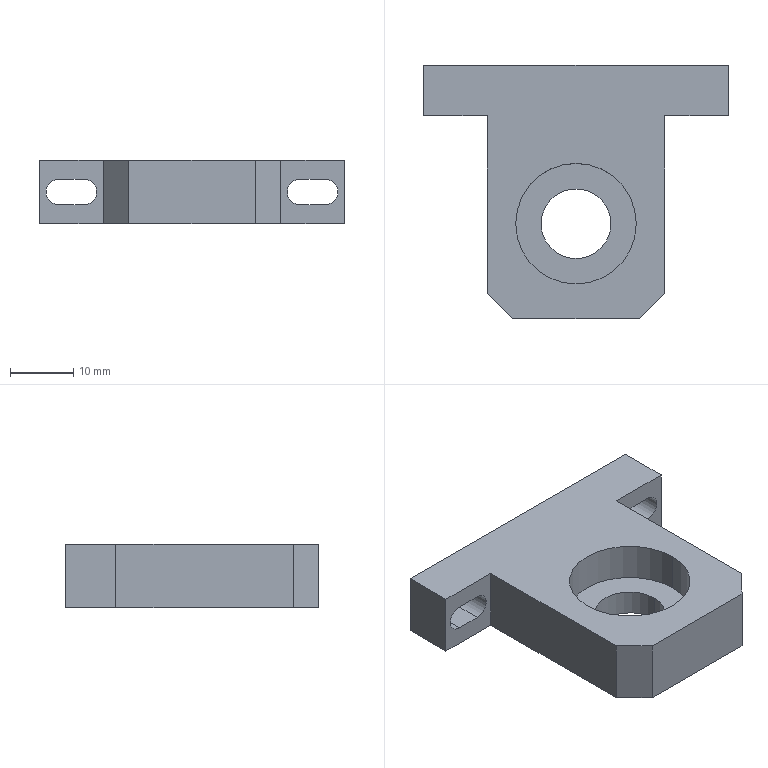Part | SolidWorks | features BaseBody 1 | 1 solid | 25 faces | box 48 x 40 x 10 mm | volume 10102 mm3 | plane 17 | cylinder 8 | commonest cylinder face diameters 4 x4 11 x2 19 x2
STEP:
#1=CARTESIAN_POINT('',(277.492,-152.944,0.));
#2=VERTEX_POINT('',#1);
#3=CARTESIAN_POINT('',(266.492,-152.944,0.));
#4=VERTEX_POINT('',#3);
#5=CARTESIAN_POINT('',(271.992,-152.944,0.));
#6=DIRECTION('',(0.,0.,-1.));
#7=DIRECTION('',(1.,0.,0.));
#8=AXIS2_PLACEMENT_3D('',#5,#6,#7);
#9=CIRCLE('',#8,5.5);
#10=EDGE_CURVE('',#2,#4,#9,.T.);
#11=ORIENTED_EDGE('',*,*,#10,.T.);
#12=CARTESIAN_POINT('',(266.492,-152.944,4.));
#13=VERTEX_POINT('',#12);
#14=CARTESIAN_POINT('',(266.492,-152.944,-47.446));
#15=DIRECTION('',(0.,0.,1.));
#16=VECTOR('',#15,1000.);
#17=LINE('',#14,#16);
#18=EDGE_CURVE('',#4,#13,#17,.T.);
#19=ORIENTED_EDGE('',*,*,#18,.T.);
#20=CARTESIAN_POINT('',(277.492,-152.944,4.));
#21=VERTEX_POINT('',#20);
#22=CARTESIAN_POINT('',(271.992,-152.944,4.));
#23=DIRECTION('',(0.,0.,-1.));
#24=DIRECTION('',(1.,0.,0.));
#25=AXIS2_PLACEMENT_3D('',#22,#23,#24);
#26=CIRCLE('',#25,5.5);
#27=EDGE_CURVE('',#21,#13,#26,.T.);
#28=ORIENTED_EDGE('',*,*,#27,.F.);
#29=CARTESIAN_POINT('',(277.492,-152.944,-47.446));
#30=DIRECTION('',(0.,0.,1.));
#31=VECTOR('',#30,1000.);
#32=LINE('',#29,#31);
#33=EDGE_CURVE('',#2,#21,#32,.T.);
#34=ORIENTED_EDGE('',*,*,#33,.F.);
#35=EDGE_LOOP('',(#11,#19,#28,#34));
#36=FACE_OUTER_BOUND('',#35,.T.);
#37=CARTESIAN_POINT('',(271.992,-152.944,-47.446));
#38=DIRECTION('',(0.,0.,1.));
#39=DIRECTION('',(1.,0.,0.));
#40=AXIS2_PLACEMENT_3D('',#37,#38,#39);
#41=CYLINDRICAL_SURFACE('',#40,5.5);
#42=ADVANCED_FACE('',(#36),#41,.F.);
#43=CARTESIAN_POINT('',(262.492,-152.944,4.));
#44=VERTEX_POINT('',#43);
#45=CARTESIAN_POINT('',(281.492,-152.944,4.));
#46=VERTEX_POINT('',#45);
#47=CARTESIAN_POINT('',(271.992,-152.944,4.));
#48=DIRECTION('',(0.,0.,1.));
#49=DIRECTION('',(1.,0.,0.));
#50=AXIS2_PLACEMENT_3D('',#47,#48,#49);
#51=CIRCLE('',#50,9.5);
#52=EDGE_CURVE('',#44,#46,#51,.T.);
#53=ORIENTED_EDGE('',*,*,#52,.F.);
#54=CARTESIAN_POINT('',(262.492,-152.944,10.));
#55=VERTEX_POINT('',#54);
#56=CARTESIAN_POINT('',(262.492,-152.944,7.));
#57=DIRECTION('',(0.,0.,1.));
#58=VECTOR('',#57,1000.);
#59=LINE('',#56,#58);
#60=EDGE_CURVE('',#44,#55,#59,.T.);
#61=ORIENTED_EDGE('',*,*,#60,.T.);
#62=CARTESIAN_POINT('',(281.492,-152.944,10.));
#63=VERTEX_POINT('',#62);
#64=CARTESIAN_POINT('',(271.992,-152.944,10.));
#65=DIRECTION('',(0.,0.,-1.));
#66=DIRECTION('',(1.,0.,0.));
#67=AXIS2_PLACEMENT_3D('',#64,#65,#66);
#68=CIRCLE('',#67,9.5);
#69=EDGE_CURVE('',#63,#55,#68,.T.);
#70=ORIENTED_EDGE('',*,*,#69,.F.);
#71=CARTESIAN_POINT('',(281.492,-152.944,7.));
#72=DIRECTION('',(0.,0.,1.));
#73=VECTOR('',#72,1000.);
#74=LINE('',#71,#73);
#75=EDGE_CURVE('',#46,#63,#74,.T.);
#76=ORIENTED_EDGE('',*,*,#75,.F.);
#77=EDGE_LOOP('',(#53,#61,#70,#76));
#78=FACE_OUTER_BOUND('',#77,.T.);
#79=CARTESIAN_POINT('',(271.992,-152.944,7.));
#80=DIRECTION('',(0.,0.,1.));
#81=DIRECTION('',(1.,0.,0.));
#82=AXIS2_PLACEMENT_3D('',#79,#80,#81);
#83=CYLINDRICAL_SURFACE('',#82,9.5);
#84=ADVANCED_FACE('',(#78),#83,.F.);
#85=ORIENTED_EDGE('',*,*,#10,.F.);
#86=CARTESIAN_POINT('',(271.992,-152.944,0.));
#87=DIRECTION('',(0.,0.,-1.));
#88=DIRECTION('',(1.,0.,0.));
#89=AXIS2_PLACEMENT_3D('',#86,#87,#88);
#90=CIRCLE('',#89,5.5);
#91=EDGE_CURVE('',#4,#2,#90,.T.);
#92=ORIENTED_EDGE('',*,*,#91,.F.);
#93=EDGE_LOOP('',(#85,#92));
#94=FACE_BOUND('',#93,.T.);
#95=CARTESIAN_POINT('',(261.992,-167.944,0.));
#96=VERTEX_POINT('',#95);
#97=CARTESIAN_POINT('',(281.992,-167.944,0.));
#98=VERTEX_POINT('',#97);
#99=CARTESIAN_POINT('',(271.992,-167.944,0.));
#100=DIRECTION('',(1.,0.,0.));
#101=VECTOR('',#100,1000.);
#102=LINE('',#99,#101);
#103=EDGE_CURVE('',#96,#98,#102,.T.);
#104=ORIENTED_EDGE('',*,*,#103,.F.);
#105=CARTESIAN_POINT('',(257.992,-163.944,0.));
#106=VERTEX_POINT('',#105);
#107=CARTESIAN_POINT('',(257.992,-163.944,0.));
#108=DIRECTION('',(0.7071,-0.7071,0.));
#109=VECTOR('',#108,1000.);
#110=LINE('',#107,#109);
#111=EDGE_CURVE('',#106,#96,#110,.T.);
#112=ORIENTED_EDGE('',*,*,#111,.F.);
#113=CARTESIAN_POINT('',(257.992,-135.944,0.));
#114=VERTEX_POINT('',#113);
#115=CARTESIAN_POINT('',(257.992,-147.944,0.));
#116=DIRECTION('',(0.,-1.,0.));
#117=VECTOR('',#116,1000.);
#118=LINE('',#115,#117);
#119=EDGE_CURVE('',#114,#106,#118,.T.);
#120=ORIENTED_EDGE('',*,*,#119,.F.);
#121=CARTESIAN_POINT('',(247.992,-135.944,0.));
#122=VERTEX_POINT('',#121);
#123=CARTESIAN_POINT('',(271.992,-135.944,0.));
#124=DIRECTION('',(1.,0.,0.));
#125=VECTOR('',#124,1000.);
#126=LINE('',#123,#125);
#127=EDGE_CURVE('',#122,#114,#126,.T.);
#128=ORIENTED_EDGE('',*,*,#127,.F.);
#129=CARTESIAN_POINT('',(247.992,-127.944,0.));
#130=VERTEX_POINT('',#129);
#131=CARTESIAN_POINT('',(247.992,-147.944,0.));
#132=DIRECTION('',(0.,-1.,0.));
#133=VECTOR('',#132,1000.);
#134=LINE('',#131,#133);
#135=EDGE_CURVE('',#130,#122,#134,.T.);
#136=ORIENTED_EDGE('',*,*,#135,.F.);
#137=CARTESIAN_POINT('',(295.992,-127.944,0.));
#138=VERTEX_POINT('',#137);
#139=CARTESIAN_POINT('',(271.992,-127.944,0.));
#140=DIRECTION('',(-1.,0.,0.));
#141=VECTOR('',#140,1000.);
#142=LINE('',#139,#141);
#143=EDGE_CURVE('',#138,#130,#142,.T.);
#144=ORIENTED_EDGE('',*,*,#143,.F.);
#145=CARTESIAN_POINT('',(295.992,-135.944,0.));
#146=VERTEX_POINT('',#145);
#147=CARTESIAN_POINT('',(295.992,-147.944,0.));
#148=DIRECTION('',(0.,1.,0.));
#149=VECTOR('',#148,1000.);
#150=LINE('',#147,#149);
#151=EDGE_CURVE('',#146,#138,#150,.T.);
#152=ORIENTED_EDGE('',*,*,#151,.F.);
#153=CARTESIAN_POINT('',(285.992,-135.944,0.));
#154=VERTEX_POINT('',#153);
#155=CARTESIAN_POINT('',(271.992,-135.944,0.));
#156=DIRECTION('',(1.,0.,0.));
#157=VECTOR('',#156,1000.);
#158=LINE('',#155,#157);
#159=EDGE_CURVE('',#154,#146,#158,.T.);
#160=ORIENTED_EDGE('',*,*,#159,.F.);
#161=CARTESIAN_POINT('',(285.992,-163.944,0.));
#162=VERTEX_POINT('',#161);
#163=CARTESIAN_POINT('',(285.992,-147.944,0.));
#164=DIRECTION('',(0.,1.,0.));
#165=VECTOR('',#164,1000.);
#166=LINE('',#163,#165);
#167=EDGE_CURVE('',#162,#154,#166,.T.);
#168=ORIENTED_EDGE('',*,*,#167,.F.);
#169=CARTESIAN_POINT('',(281.992,-167.944,0.));
#170=DIRECTION('',(0.7071,0.7071,0.));
#171=VECTOR('',#170,1000.);
#172=LINE('',#169,#171);
#173=EDGE_CURVE('',#98,#162,#172,.T.);
#174=ORIENTED_EDGE('',*,*,#173,.F.);
#175=EDGE_LOOP('',(#104,#112,#120,#128,#136,#144,#152,#160,#168,#174));
#176=FACE_OUTER_BOUND('',#175,.T.);
#177=CARTESIAN_POINT('',(271.992,-147.944,0.));
#178=DIRECTION('',(0.,0.,1.));
#179=DIRECTION('',(1.,0.,0.));
#180=AXIS2_PLACEMENT_3D('',#177,#178,#179);
#181=PLANE('',#180);
#182=ADVANCED_FACE('',(#94,#176),#181,.F.);
#183=ORIENTED_EDGE('',*,*,#18,.F.);
#184=ORIENTED_EDGE('',*,*,#91,.T.);
#185=ORIENTED_EDGE('',*,*,#33,.T.);
#186=CARTESIAN_POINT('',(271.992,-152.944,4.));
#187=DIRECTION('',(0.,0.,-1.));
#188=DIRECTION('',(1.,0.,0.));
#189=AXIS2_PLACEMENT_3D('',#186,#187,#188);
#190=CIRCLE('',#189,5.5);
#191=EDGE_CURVE('',#13,#21,#190,.T.);
#192=ORIENTED_EDGE('',*,*,#191,.F.);
#193=EDGE_LOOP('',(#183,#184,#185,#192));
#194=FACE_OUTER_BOUND('',#193,.T.);
#195=CARTESIAN_POINT('',(271.992,-152.944,-47.446));
#196=DIRECTION('',(0.,0.,1.));
#197=DIRECTION('',(1.,0.,0.));
#198=AXIS2_PLACEMENT_3D('',#195,#196,#197);
#199=CYLINDRICAL_SURFACE('',#198,5.5);
#200=ADVANCED_FACE('',(#194),#199,.F.);
#201=ORIENTED_EDGE('',*,*,#173,.T.);
#202=CARTESIAN_POINT('',(285.992,-163.944,10.));
#203=VERTEX_POINT('',#202);
#204=CARTESIAN_POINT('',(285.992,-163.944,5.));
#205=DIRECTION('',(0.,0.,1.));
#206=VECTOR('',#205,1000.);
#207=LINE('',#204,#206);
#208=EDGE_CURVE('',#162,#203,#207,.T.);
#209=ORIENTED_EDGE('',*,*,#208,.T.);
#210=CARTESIAN_POINT('',(281.992,-167.944,10.));
#211=VERTEX_POINT('',#210);
#212=CARTESIAN_POINT('',(283.992,-165.944,10.));
#213=DIRECTION('',(-0.7071,-0.7071,0.));
#214=VECTOR('',#213,1000.);
#215=LINE('',#212,#214);
#216=EDGE_CURVE('',#203,#211,#215,.T.);
#217=ORIENTED_EDGE('',*,*,#216,.T.);
#218=CARTESIAN_POINT('',(281.992,-167.944,5.));
#219=DIRECTION('',(0.,0.,-1.));
#220=VECTOR('',#219,1000.);
#221=LINE('',#218,#220);
#222=EDGE_CURVE('',#211,#98,#221,.T.);
#223=ORIENTED_EDGE('',*,*,#222,.T.);
#224=EDGE_LOOP('',(#201,#209,#217,#223));
#225=FACE_OUTER_BOUND('',#224,.T.);
#226=CARTESIAN_POINT('',(283.992,-165.944,5.));
#227=DIRECTION('',(0.7071,-0.7071,0.));
#228=DIRECTION('',(0.7071,0.7071,0.));
#229=AXIS2_PLACEMENT_3D('',#226,#227,#228);
#230=PLANE('',#229);
#231=ADVANCED_FACE('',(#225),#230,.T.);
#232=CARTESIAN_POINT('',(261.992,-167.944,10.));
#233=VERTEX_POINT('',#232);
#234=CARTESIAN_POINT('',(261.992,-167.944,0.));
#235=DIRECTION('',(0.,0.,-1.));
#236=VECTOR('',#235,1000.);
#237=LINE('',#234,#236);
#238=EDGE_CURVE('',#233,#96,#237,.T.);
#239=ORIENTED_EDGE('',*,*,#238,.T.);
#240=ORIENTED_EDGE('',*,*,#103,.T.);
#241=ORIENTED_EDGE('',*,*,#222,.F.);
#242=CARTESIAN_POINT('',(291.992,-167.944,10.));
#243=DIRECTION('',(-1.,0.,0.));
#244=VECTOR('',#243,1000.);
#245=LINE('',#242,#244);
#246=EDGE_CURVE('',#211,#233,#245,.T.);
#247=ORIENTED_EDGE('',*,*,#246,.T.);
#248=EDGE_LOOP('',(#239,#240,#241,#247));
#249=FACE_OUTER_BOUND('',#248,.T.);
#250=CARTESIAN_POINT('',(291.992,-167.944,0.));
#251=DIRECTION('',(0.,-1.,0.));
#252=DIRECTION('',(0.,0.,-1.));
#253=AXIS2_PLACEMENT_3D('',#250,#251,#252);
#254=PLANE('',#253);
#255=ADVANCED_FACE('',(#249),#254,.T.);
#256=CARTESIAN_POINT('',(257.992,-163.944,10.));
#257=VERTEX_POINT('',#256);
#258=CARTESIAN_POINT('',(259.992,-165.944,10.));
#259=DIRECTION('',(-0.7071,0.7071,0.));
#260=VECTOR('',#259,1000.);
#261=LINE('',#258,#260);
#262=EDGE_CURVE('',#233,#257,#261,.T.);
#263=ORIENTED_EDGE('',*,*,#262,.T.);
#264=CARTESIAN_POINT('',(257.992,-163.944,5.));
#265=DIRECTION('',(0.,0.,-1.));
#266=VECTOR('',#265,1000.);
#267=LINE('',#264,#266);
#268=EDGE_CURVE('',#257,#106,#267,.T.);
#269=ORIENTED_EDGE('',*,*,#268,.T.);
#270=ORIENTED_EDGE('',*,*,#111,.T.);
#271=ORIENTED_EDGE('',*,*,#238,.F.);
#272=EDGE_LOOP('',(#263,#269,#270,#271));
#273=FACE_OUTER_BOUND('',#272,.T.);
#274=CARTESIAN_POINT('',(259.992,-165.944,5.));
#275=DIRECTION('',(-0.7071,-0.7071,0.));
#276=DIRECTION('',(0.7071,-0.7071,0.));
#277=AXIS2_PLACEMENT_3D('',#274,#275,#276);
#278=PLANE('',#277);
#279=ADVANCED_FACE('',(#273),#278,.T.);
#280=CARTESIAN_POINT('',(257.992,-135.944,10.));
#281=VERTEX_POINT('',#280);
#282=CARTESIAN_POINT('',(257.992,-167.944,10.));
#283=DIRECTION('',(0.,-1.,0.));
#284=VECTOR('',#283,1000.);
#285=LINE('',#282,#284);
#286=EDGE_CURVE('',#281,#257,#285,.T.);
#287=ORIENTED_EDGE('',*,*,#286,.F.);
#288=CARTESIAN_POINT('',(257.992,-135.944,10.));
#289=DIRECTION('',(0.,0.,1.));
#290=VECTOR('',#289,1000.);
#291=LINE('',#288,#290);
#292=EDGE_CURVE('',#114,#281,#291,.T.);
#293=ORIENTED_EDGE('',*,*,#292,.F.);
#294=ORIENTED_EDGE('',*,*,#119,.T.);
#295=ORIENTED_EDGE('',*,*,#268,.F.);
#296=EDGE_LOOP('',(#287,#293,#294,#295));
#297=FACE_OUTER_BOUND('',#296,.T.);
#298=CARTESIAN_POINT('',(257.992,-167.944,10.));
#299=DIRECTION('',(1.,0.,0.));
#300=DIRECTION('',(0.,0.,-1.));
#301=AXIS2_PLACEMENT_3D('',#298,#299,#300);
#302=PLANE('',#301);
#303=ADVANCED_FACE('',(#297),#302,.F.);
#304=CARTESIAN_POINT('',(250.992,-135.944,3.));
#305=VERTEX_POINT('',#304);
#306=CARTESIAN_POINT('',(254.992,-135.944,3.));
#307=VERTEX_POINT('',#306);
#308=CARTESIAN_POINT('',(257.992,-135.944,3.));
#309=DIRECTION('',(1.,0.,0.));
#310=VECTOR('',#309,1000.);
#311=LINE('',#308,#310);
#312=EDGE_CURVE('',#305,#307,#311,.T.);
#313=ORIENTED_EDGE('',*,*,#312,.F.);
#314=CARTESIAN_POINT('',(250.992,-135.944,7.));
#315=VERTEX_POINT('',#314);
#316=CARTESIAN_POINT('',(250.992,-135.944,5.));
#317=DIRECTION('',(0.,-1.,0.));
#318=DIRECTION('',(0.,0.,1.));
#319=AXIS2_PLACEMENT_3D('',#316,#317,#318);
#320=CIRCLE('',#319,2.);
#321=EDGE_CURVE('',#315,#305,#320,.T.);
#322=ORIENTED_EDGE('',*,*,#321,.F.);
#323=CARTESIAN_POINT('',(254.992,-135.944,7.));
#324=VERTEX_POINT('',#323);
#325=CARTESIAN_POINT('',(257.992,-135.944,7.));
#326=DIRECTION('',(-1.,0.,0.));
#327=VECTOR('',#326,1000.);
#328=LINE('',#325,#327);
#329=EDGE_CURVE('',#324,#315,#328,.T.);
#330=ORIENTED_EDGE('',*,*,#329,.F.);
#331=CARTESIAN_POINT('',(254.992,-135.944,5.));
#332=DIRECTION('',(0.,-1.,0.));
#333=DIRECTION('',(0.,0.,1.));
#334=AXIS2_PLACEMENT_3D('',#331,#332,#333);
#335=CIRCLE('',#334,2.);
#336=EDGE_CURVE('',#307,#324,#335,.T.);
#337=ORIENTED_EDGE('',*,*,#336,.F.);
#338=EDGE_LOOP('',(#313,#322,#330,#337));
#339=FACE_BOUND('',#338,.T.);
#340=ORIENTED_EDGE('',*,*,#292,.T.);
#341=CARTESIAN_POINT('',(247.992,-135.944,10.));
#342=VERTEX_POINT('',#341);
#343=CARTESIAN_POINT('',(257.992,-135.944,10.));
#344=DIRECTION('',(1.,0.,0.));
#345=VECTOR('',#344,1000.);
#346=LINE('',#343,#345);
#347=EDGE_CURVE('',#342,#281,#346,.T.);
#348=ORIENTED_EDGE('',*,*,#347,.F.);
#349=CARTESIAN_POINT('',(247.992,-135.944,10.));
#350=DIRECTION('',(0.,0.,1.));
#351=VECTOR('',#350,1000.);
#352=LINE('',#349,#351);
#353=EDGE_CURVE('',#122,#342,#352,.T.);
#354=ORIENTED_EDGE('',*,*,#353,.F.);
#355=ORIENTED_EDGE('',*,*,#127,.T.);
#356=EDGE_LOOP('',(#340,#348,#354,#355));
#357=FACE_OUTER_BOUND('',#356,.T.);
#358=CARTESIAN_POINT('',(257.992,-135.944,10.));
#359=DIRECTION('',(0.,1.,0.));
#360=DIRECTION('',(0.,0.,1.));
#361=AXIS2_PLACEMENT_3D('',#358,#359,#360);
#362=PLANE('',#361);
#363=ADVANCED_FACE('',(#339,#357),#362,.F.);
#364=ORIENTED_EDGE('',*,*,#353,.T.);
#365=CARTESIAN_POINT('',(247.992,-127.944,10.));
#366=VERTEX_POINT('',#365);
#367=CARTESIAN_POINT('',(247.992,-131.944,10.));
#368=DIRECTION('',(0.,-1.,0.));
#369=VECTOR('',#368,1000.);
#370=LINE('',#367,#369);
#371=EDGE_CURVE('',#366,#342,#370,.T.);
#372=ORIENTED_EDGE('',*,*,#371,.F.);
#373=CARTESIAN_POINT('',(247.992,-127.944,5.));
#374=DIRECTION('',(0.,0.,1.));
#375=VECTOR('',#374,1000.);
#376=LINE('',#373,#375);
#377=EDGE_CURVE('',#130,#366,#376,.T.);
#378=ORIENTED_EDGE('',*,*,#377,.F.);
#379=ORIENTED_EDGE('',*,*,#135,.T.);
#380=EDGE_LOOP('',(#364,#372,#378,#379));
#381=FACE_OUTER_BOUND('',#380,.T.);
#382=CARTESIAN_POINT('',(247.992,-131.944,5.));
#383=DIRECTION('',(1.,0.,0.));
#384=DIRECTION('',(0.,0.,-1.));
#385=AXIS2_PLACEMENT_3D('',#382,#383,#384);
#386=PLANE('',#385);
#387=ADVANCED_FACE('',(#381),#386,.F.);
#388=CARTESIAN_POINT('',(250.992,-127.944,7.));
#389=VERTEX_POINT('',#388);
#390=CARTESIAN_POINT('',(250.992,-127.944,3.));
#391=VERTEX_POINT('',#390);
#392=CARTESIAN_POINT('',(250.992,-127.944,5.));
#393=DIRECTION('',(0.,-1.,0.));
#394=DIRECTION('',(0.,0.,1.));
#395=AXIS2_PLACEMENT_3D('',#392,#393,#394);
#396=CIRCLE('',#395,2.);
#397=EDGE_CURVE('',#389,#391,#396,.T.);
#398=ORIENTED_EDGE('',*,*,#397,.T.);
#399=CARTESIAN_POINT('',(254.992,-127.944,3.));
#400=VERTEX_POINT('',#399);
#401=CARTESIAN_POINT('',(251.992,-127.944,3.));
#402=DIRECTION('',(1.,0.,0.));
#403=VECTOR('',#402,1000.);
#404=LINE('',#401,#403);
#405=EDGE_CURVE('',#391,#400,#404,.T.);
#406=ORIENTED_EDGE('',*,*,#405,.T.);
#407=CARTESIAN_POINT('',(254.992,-127.944,7.));
#408=VERTEX_POINT('',#407);
#409=CARTESIAN_POINT('',(254.992,-127.944,5.));
#410=DIRECTION('',(0.,-1.,0.));
#411=DIRECTION('',(0.,0.,1.));
#412=AXIS2_PLACEMENT_3D('',#409,#410,#411);
#413=CIRCLE('',#412,2.);
#414=EDGE_CURVE('',#400,#408,#413,.T.);
#415=ORIENTED_EDGE('',*,*,#414,.T.);
#416=CARTESIAN_POINT('',(251.992,-127.944,7.));
#417=DIRECTION('',(-1.,0.,0.));
#418=VECTOR('',#417,1000.);
#419=LINE('',#416,#418);
#420=EDGE_CURVE('',#408,#389,#419,.T.);
#421=ORIENTED_EDGE('',*,*,#420,.T.);
#422=EDGE_LOOP('',(#398,#406,#415,#421));
#423=FACE_BOUND('',#422,.T.);
#424=CARTESIAN_POINT('',(288.992,-127.944,7.));
#425=VERTEX_POINT('',#424);
#426=CARTESIAN_POINT('',(288.992,-127.944,3.));
#427=VERTEX_POINT('',#426);
#428=CARTESIAN_POINT('',(288.992,-127.944,5.));
#429=DIRECTION('',(0.,-1.,0.));
#430=DIRECTION('',(0.,0.,1.));
#431=AXIS2_PLACEMENT_3D('',#428,#429,#430);
#432=CIRCLE('',#431,2.);
#433=EDGE_CURVE('',#425,#427,#432,.T.);
#434=ORIENTED_EDGE('',*,*,#433,.T.);
#435=CARTESIAN_POINT('',(292.992,-127.944,3.));
#436=VERTEX_POINT('',#435);
#437=CARTESIAN_POINT('',(251.992,-127.944,3.));
#438=DIRECTION('',(1.,0.,0.));
#439=VECTOR('',#438,1000.);
#440=LINE('',#437,#439);
#441=EDGE_CURVE('',#427,#436,#440,.T.);
#442=ORIENTED_EDGE('',*,*,#441,.T.);
#443=CARTESIAN_POINT('',(292.992,-127.944,7.));
#444=VERTEX_POINT('',#443);
#445=CARTESIAN_POINT('',(292.992,-127.944,5.));
#446=DIRECTION('',(0.,-1.,0.));
#447=DIRECTION('',(0.,0.,1.));
#448=AXIS2_PLACEMENT_3D('',#445,#446,#447);
#449=CIRCLE('',#448,2.);
#450=EDGE_CURVE('',#436,#444,#449,.T.);
#451=ORIENTED_EDGE('',*,*,#450,.T.);
#452=CARTESIAN_POINT('',(251.992,-127.944,7.));
#453=DIRECTION('',(-1.,0.,0.));
#454=VECTOR('',#453,1000.);
#455=LINE('',#452,#454);
#456=EDGE_CURVE('',#444,#425,#455,.T.);
#457=ORIENTED_EDGE('',*,*,#456,.T.);
#458=EDGE_LOOP('',(#434,#442,#451,#457));
#459=FACE_BOUND('',#458,.T.);
#460=ORIENTED_EDGE('',*,*,#143,.T.);
#461=ORIENTED_EDGE('',*,*,#377,.T.);
#462=CARTESIAN_POINT('',(295.992,-127.944,10.));
#463=VERTEX_POINT('',#462);
#464=CARTESIAN_POINT('',(251.992,-127.944,10.));
#465=DIRECTION('',(1.,0.,0.));
#466=VECTOR('',#465,1000.);
#467=LINE('',#464,#466);
#468=EDGE_CURVE('',#366,#463,#467,.T.);
#469=ORIENTED_EDGE('',*,*,#468,.T.);
#470=CARTESIAN_POINT('',(295.992,-127.944,0.));
#471=DIRECTION('',(0.,0.,-1.));
#472=VECTOR('',#471,1000.);
#473=LINE('',#470,#472);
#474=EDGE_CURVE('',#463,#138,#473,.T.);
#475=ORIENTED_EDGE('',*,*,#474,.T.);
#476=EDGE_LOOP('',(#460,#461,#469,#475));
#477=FACE_OUTER_BOUND('',#476,.T.);
#478=CARTESIAN_POINT('',(251.992,-127.944,0.));
#479=DIRECTION('',(0.,1.,0.));
#480=DIRECTION('',(0.,0.,1.));
#481=AXIS2_PLACEMENT_3D('',#478,#479,#480);
#482=PLANE('',#481);
#483=ADVANCED_FACE('',(#423,#459,#477),#482,.T.);
#484=ORIENTED_EDGE('',*,*,#151,.T.);
#485=ORIENTED_EDGE('',*,*,#474,.F.);
#486=CARTESIAN_POINT('',(295.992,-135.944,10.));
#487=VERTEX_POINT('',#486);
#488=CARTESIAN_POINT('',(295.992,-131.944,10.));
#489=DIRECTION('',(0.,-1.,0.));
#490=VECTOR('',#489,1000.);
#491=LINE('',#488,#490);
#492=EDGE_CURVE('',#463,#487,#491,.T.);
#493=ORIENTED_EDGE('',*,*,#492,.T.);
#494=CARTESIAN_POINT('',(295.992,-135.944,5.));
#495=DIRECTION('',(0.,0.,-1.));
#496=VECTOR('',#495,1000.);
#497=LINE('',#494,#496);
#498=EDGE_CURVE('',#487,#146,#497,.T.);
#499=ORIENTED_EDGE('',*,*,#498,.T.);
#500=EDGE_LOOP('',(#484,#485,#493,#499));
#501=FACE_OUTER_BOUND('',#500,.T.);
#502=CARTESIAN_POINT('',(295.992,-131.944,5.));
#503=DIRECTION('',(1.,0.,0.));
#504=DIRECTION('',(0.,0.,-1.));
#505=AXIS2_PLACEMENT_3D('',#502,#503,#504);
#506=PLANE('',#505);
#507=ADVANCED_FACE('',(#501),#506,.T.);
#508=CARTESIAN_POINT('',(288.992,-135.944,3.));
#509=VERTEX_POINT('',#508);
#510=CARTESIAN_POINT('',(292.992,-135.944,3.));
#511=VERTEX_POINT('',#510);
#512=CARTESIAN_POINT('',(291.992,-135.944,3.));
#513=DIRECTION('',(1.,0.,0.));
#514=VECTOR('',#513,1000.);
#515=LINE('',#512,#514);
#516=EDGE_CURVE('',#509,#511,#515,.T.);
#517=ORIENTED_EDGE('',*,*,#516,.F.);
#518=CARTESIAN_POINT('',(288.992,-135.944,7.));
#519=VERTEX_POINT('',#518);
#520=CARTESIAN_POINT('',(288.992,-135.944,5.));
#521=DIRECTION('',(0.,-1.,0.));
#522=DIRECTION('',(0.,0.,1.));
#523=AXIS2_PLACEMENT_3D('',#520,#521,#522);
#524=CIRCLE('',#523,2.);
#525=EDGE_CURVE('',#519,#509,#524,.T.);
#526=ORIENTED_EDGE('',*,*,#525,.F.);
#527=CARTESIAN_POINT('',(292.992,-135.944,7.));
#528=VERTEX_POINT('',#527);
#529=CARTESIAN_POINT('',(291.992,-135.944,7.));
#530=DIRECTION('',(-1.,0.,0.));
#531=VECTOR('',#530,1000.);
#532=LINE('',#529,#531);
#533=EDGE_CURVE('',#528,#519,#532,.T.);
#534=ORIENTED_EDGE('',*,*,#533,.F.);
#535=CARTESIAN_POINT('',(292.992,-135.944,5.));
#536=DIRECTION('',(0.,-1.,0.));
#537=DIRECTION('',(0.,0.,1.));
#538=AXIS2_PLACEMENT_3D('',#535,#536,#537);
#539=CIRCLE('',#538,2.);
#540=EDGE_CURVE('',#511,#528,#539,.T.);
#541=ORIENTED_EDGE('',*,*,#540,.F.);
#542=EDGE_LOOP('',(#517,#526,#534,#541));
#543=FACE_BOUND('',#542,.T.);
#544=ORIENTED_EDGE('',*,*,#498,.F.);
#545=CARTESIAN_POINT('',(285.992,-135.944,10.));
#546=VERTEX_POINT('',#545);
#547=CARTESIAN_POINT('',(291.992,-135.944,10.));
#548=DIRECTION('',(1.,0.,0.));
#549=VECTOR('',#548,1000.);
#550=LINE('',#547,#549);
#551=EDGE_CURVE('',#546,#487,#550,.T.);
#552=ORIENTED_EDGE('',*,*,#551,.F.);
#553=CARTESIAN_POINT('',(285.992,-135.944,10.));
#554=DIRECTION('',(0.,0.,1.));
#555=VECTOR('',#554,1000.);
#556=LINE('',#553,#555);
#557=EDGE_CURVE('',#154,#546,#556,.T.);
#558=ORIENTED_EDGE('',*,*,#557,.F.);
#559=ORIENTED_EDGE('',*,*,#159,.T.);
#560=EDGE_LOOP('',(#544,#552,#558,#559));
#561=FACE_OUTER_BOUND('',#560,.T.);
#562=CARTESIAN_POINT('',(291.992,-135.944,10.));
#563=DIRECTION('',(0.,1.,0.));
#564=DIRECTION('',(0.,0.,1.));
#565=AXIS2_PLACEMENT_3D('',#562,#563,#564);
#566=PLANE('',#565);
#567=ADVANCED_FACE('',(#543,#561),#566,.F.);
#568=ORIENTED_EDGE('',*,*,#167,.T.);
#569=ORIENTED_EDGE('',*,*,#557,.T.);
#570=CARTESIAN_POINT('',(285.992,-135.944,10.));
#571=DIRECTION('',(0.,1.,0.));
#572=VECTOR('',#571,1000.);
#573=LINE('',#570,#572);
#574=EDGE_CURVE('',#203,#546,#573,.T.);
#575=ORIENTED_EDGE('',*,*,#574,.F.);
#576=ORIENTED_EDGE('',*,*,#208,.F.);
#577=EDGE_LOOP('',(#568,#569,#575,#576));
#578=FACE_OUTER_BOUND('',#577,.T.);
#579=CARTESIAN_POINT('',(285.992,-135.944,10.));
#580=DIRECTION('',(-1.,0.,0.));
#581=DIRECTION('',(0.,0.,1.));
#582=AXIS2_PLACEMENT_3D('',#579,#580,#581);
#583=PLANE('',#582);
#584=ADVANCED_FACE('',(#578),#583,.F.);
#585=ORIENTED_EDGE('',*,*,#27,.T.);
#586=ORIENTED_EDGE('',*,*,#191,.T.);
#587=EDGE_LOOP('',(#585,#586));
#588=FACE_BOUND('',#587,.T.);
#589=CARTESIAN_POINT('',(271.992,-152.944,4.));
#590=DIRECTION('',(0.,0.,1.));
#591=DIRECTION('',(1.,0.,0.));
#592=AXIS2_PLACEMENT_3D('',#589,#590,#591);
#593=CIRCLE('',#592,9.5);
#594=EDGE_CURVE('',#46,#44,#593,.T.);
#595=ORIENTED_EDGE('',*,*,#594,.T.);
#596=ORIENTED_EDGE('',*,*,#52,.T.);
#597=EDGE_LOOP('',(#595,#596));
#598=FACE_OUTER_BOUND('',#597,.T.);
#599=CARTESIAN_POINT('',(271.992,-152.944,4.));
#600=DIRECTION('',(0.,0.,1.));
#601=DIRECTION('',(1.,0.,0.));
#602=AXIS2_PLACEMENT_3D('',#599,#600,#601);
#603=PLANE('',#602);
#604=ADVANCED_FACE('',(#588,#598),#603,.T.);
#605=ORIENTED_EDGE('',*,*,#69,.T.);
#606=CARTESIAN_POINT('',(271.992,-152.944,10.));
#607=DIRECTION('',(0.,0.,-1.));
#608=DIRECTION('',(1.,0.,0.));
#609=AXIS2_PLACEMENT_3D('',#606,#607,#608);
#610=CIRCLE('',#609,9.5);
#611=EDGE_CURVE('',#55,#63,#610,.T.);
#612=ORIENTED_EDGE('',*,*,#611,.T.);
#613=EDGE_LOOP('',(#605,#612));
#614=FACE_BOUND('',#613,.T.);
#615=ORIENTED_EDGE('',*,*,#262,.F.);
#616=ORIENTED_EDGE('',*,*,#246,.F.);
#617=ORIENTED_EDGE('',*,*,#216,.F.);
#618=ORIENTED_EDGE('',*,*,#574,.T.);
#619=ORIENTED_EDGE('',*,*,#551,.T.);
#620=ORIENTED_EDGE('',*,*,#492,.F.);
#621=ORIENTED_EDGE('',*,*,#468,.F.);
#622=ORIENTED_EDGE('',*,*,#371,.T.);
#623=ORIENTED_EDGE('',*,*,#347,.T.);
#624=ORIENTED_EDGE('',*,*,#286,.T.);
#625=EDGE_LOOP('',(#615,#616,#617,#618,#619,#620,#621,#622,#623,#624));
#626=FACE_OUTER_BOUND('',#625,.T.);
#627=CARTESIAN_POINT('',(271.992,-147.944,10.));
#628=DIRECTION('',(0.,0.,1.));
#629=DIRECTION('',(1.,0.,0.));
#630=AXIS2_PLACEMENT_3D('',#627,#628,#629);
#631=PLANE('',#630);
#632=ADVANCED_FACE('',(#614,#626),#631,.T.);
#633=CARTESIAN_POINT('',(254.992,-135.944,3.));
#634=DIRECTION('',(0.,1.,0.));
#635=VECTOR('',#634,1000.);
#636=LINE('',#633,#635);
#637=EDGE_CURVE('',#307,#400,#636,.T.);
#638=ORIENTED_EDGE('',*,*,#637,.F.);
#639=ORIENTED_EDGE('',*,*,#336,.T.);
#640=CARTESIAN_POINT('',(254.992,-135.944,7.));
#641=DIRECTION('',(0.,-1.,0.));
#642=VECTOR('',#641,1000.);
#643=LINE('',#640,#642);
#644=EDGE_CURVE('',#408,#324,#643,.T.);
#645=ORIENTED_EDGE('',*,*,#644,.F.);
#646=ORIENTED_EDGE('',*,*,#414,.F.);
#647=EDGE_LOOP('',(#638,#639,#645,#646));
#648=FACE_OUTER_BOUND('',#647,.T.);
#649=CARTESIAN_POINT('',(254.992,-135.944,5.));
#650=DIRECTION('',(0.,1.,0.));
#651=DIRECTION('',(0.,0.,1.));
#652=AXIS2_PLACEMENT_3D('',#649,#650,#651);
#653=CYLINDRICAL_SURFACE('',#652,2.);
#654=ADVANCED_FACE('',(#648),#653,.F.);
#655=CARTESIAN_POINT('',(250.992,-135.944,3.));
#656=DIRECTION('',(0.,1.,0.));
#657=VECTOR('',#656,1000.);
#658=LINE('',#655,#657);
#659=EDGE_CURVE('',#305,#391,#658,.T.);
#660=ORIENTED_EDGE('',*,*,#659,.F.);
#661=ORIENTED_EDGE('',*,*,#312,.T.);
#662=ORIENTED_EDGE('',*,*,#637,.T.);
#663=ORIENTED_EDGE('',*,*,#405,.F.);
#664=EDGE_LOOP('',(#660,#661,#662,#663));
#665=FACE_OUTER_BOUND('',#664,.T.);
#666=CARTESIAN_POINT('',(250.992,-135.944,3.));
#667=DIRECTION('',(0.,0.,-1.));
#668=DIRECTION('',(-1.,0.,0.));
#669=AXIS2_PLACEMENT_3D('',#666,#667,#668);
#670=PLANE('',#669);
#671=ADVANCED_FACE('',(#665),#670,.F.);
#672=CARTESIAN_POINT('',(250.992,-135.944,7.));
#673=DIRECTION('',(0.,1.,0.));
#674=VECTOR('',#673,1000.);
#675=LINE('',#672,#674);
#676=EDGE_CURVE('',#315,#389,#675,.T.);
#677=ORIENTED_EDGE('',*,*,#676,.F.);
#678=ORIENTED_EDGE('',*,*,#321,.T.);
#679=ORIENTED_EDGE('',*,*,#659,.T.);
#680=ORIENTED_EDGE('',*,*,#397,.F.);
#681=EDGE_LOOP('',(#677,#678,#679,#680));
#682=FACE_OUTER_BOUND('',#681,.T.);
#683=CARTESIAN_POINT('',(250.992,-135.944,5.));
#684=DIRECTION('',(0.,1.,0.));
#685=DIRECTION('',(0.,0.,1.));
#686=AXIS2_PLACEMENT_3D('',#683,#684,#685);
#687=CYLINDRICAL_SURFACE('',#686,2.);
#688=ADVANCED_FACE('',(#682),#687,.F.);
#689=ORIENTED_EDGE('',*,*,#644,.T.);
#690=ORIENTED_EDGE('',*,*,#329,.T.);
#691=ORIENTED_EDGE('',*,*,#676,.T.);
#692=ORIENTED_EDGE('',*,*,#420,.F.);
#693=EDGE_LOOP('',(#689,#690,#691,#692));
#694=FACE_OUTER_BOUND('',#693,.T.);
#695=CARTESIAN_POINT('',(254.992,-135.944,7.));
#696=DIRECTION('',(0.,0.,1.));
#697=DIRECTION('',(1.,0.,0.));
#698=AXIS2_PLACEMENT_3D('',#695,#696,#697);
#699=PLANE('',#698);
#700=ADVANCED_FACE('',(#694),#699,.F.);
#701=CARTESIAN_POINT('',(288.992,-135.944,3.));
#702=DIRECTION('',(0.,1.,0.));
#703=VECTOR('',#702,1000.);
#704=LINE('',#701,#703);
#705=EDGE_CURVE('',#509,#427,#704,.T.);
#706=ORIENTED_EDGE('',*,*,#705,.F.);
#707=ORIENTED_EDGE('',*,*,#516,.T.);
#708=CARTESIAN_POINT('',(292.992,-135.944,3.));
#709=DIRECTION('',(0.,-1.,0.));
#710=VECTOR('',#709,1000.);
#711=LINE('',#708,#710);
#712=EDGE_CURVE('',#436,#511,#711,.T.);
#713=ORIENTED_EDGE('',*,*,#712,.F.);
#714=ORIENTED_EDGE('',*,*,#441,.F.);
#715=EDGE_LOOP('',(#706,#707,#713,#714));
#716=FACE_OUTER_BOUND('',#715,.T.);
#717=CARTESIAN_POINT('',(288.992,-135.944,3.));
#718=DIRECTION('',(0.,0.,-1.));
#719=DIRECTION('',(-1.,0.,0.));
#720=AXIS2_PLACEMENT_3D('',#717,#718,#719);
#721=PLANE('',#720);
#722=ADVANCED_FACE('',(#716),#721,.F.);
#723=CARTESIAN_POINT('',(288.992,-135.944,7.));
#724=DIRECTION('',(0.,1.,0.));
#725=VECTOR('',#724,1000.);
#726=LINE('',#723,#725);
#727=EDGE_CURVE('',#519,#425,#726,.T.);
#728=ORIENTED_EDGE('',*,*,#727,.F.);
#729=ORIENTED_EDGE('',*,*,#525,.T.);
#730=ORIENTED_EDGE('',*,*,#705,.T.);
#731=ORIENTED_EDGE('',*,*,#433,.F.);
#732=EDGE_LOOP('',(#728,#729,#730,#731));
#733=FACE_OUTER_BOUND('',#732,.T.);
#734=CARTESIAN_POINT('',(288.992,-135.944,5.));
#735=DIRECTION('',(0.,1.,0.));
#736=DIRECTION('',(0.,0.,1.));
#737=AXIS2_PLACEMENT_3D('',#734,#735,#736);
#738=CYLINDRICAL_SURFACE('',#737,2.);
#739=ADVANCED_FACE('',(#733),#738,.F.);
#740=CARTESIAN_POINT('',(292.992,-135.944,7.));
#741=DIRECTION('',(0.,1.,0.));
#742=VECTOR('',#741,1000.);
#743=LINE('',#740,#742);
#744=EDGE_CURVE('',#528,#444,#743,.T.);
#745=ORIENTED_EDGE('',*,*,#744,.F.);
#746=ORIENTED_EDGE('',*,*,#533,.T.);
#747=ORIENTED_EDGE('',*,*,#727,.T.);
#748=ORIENTED_EDGE('',*,*,#456,.F.);
#749=EDGE_LOOP('',(#745,#746,#747,#748));
#750=FACE_OUTER_BOUND('',#749,.T.);
#751=CARTESIAN_POINT('',(292.992,-135.944,7.));
#752=DIRECTION('',(0.,0.,1.));
#753=DIRECTION('',(1.,0.,0.));
#754=AXIS2_PLACEMENT_3D('',#751,#752,#753);
#755=PLANE('',#754);
#756=ADVANCED_FACE('',(#750),#755,.F.);
#757=ORIENTED_EDGE('',*,*,#712,.T.);
#758=ORIENTED_EDGE('',*,*,#540,.T.);
#759=ORIENTED_EDGE('',*,*,#744,.T.);
#760=ORIENTED_EDGE('',*,*,#450,.F.);
#761=EDGE_LOOP('',(#757,#758,#759,#760));
#762=FACE_OUTER_BOUND('',#761,.T.);
#763=CARTESIAN_POINT('',(292.992,-135.944,5.));
#764=DIRECTION('',(0.,1.,0.));
#765=DIRECTION('',(0.,0.,1.));
#766=AXIS2_PLACEMENT_3D('',#763,#764,#765);
#767=CYLINDRICAL_SURFACE('',#766,2.);
#768=ADVANCED_FACE('',(#762),#767,.F.);
#769=ORIENTED_EDGE('',*,*,#60,.F.);
#770=ORIENTED_EDGE('',*,*,#594,.F.);
#771=ORIENTED_EDGE('',*,*,#75,.T.);
#772=ORIENTED_EDGE('',*,*,#611,.F.);
#773=EDGE_LOOP('',(#769,#770,#771,#772));
#774=FACE_OUTER_BOUND('',#773,.T.);
#775=CARTESIAN_POINT('',(271.992,-152.944,7.));
#776=DIRECTION('',(0.,0.,1.));
#777=DIRECTION('',(1.,0.,0.));
#778=AXIS2_PLACEMENT_3D('',#775,#776,#777);
#779=CYLINDRICAL_SURFACE('',#778,9.5);
#780=ADVANCED_FACE('',(#774),#779,.F.);
#781=CLOSED_SHELL('',(#42,#84,#182,#200,#231,#255,#279,#303,#363,#387,#483,#507,#567,#584,#604,#632,#654,#671,#688,#700,#722,#739,#756,#768,#780));
#782=MANIFOLD_SOLID_BREP('',#781);
#783=CARTESIAN_POINT('',(0.,0.,0.));
#784=DIRECTION('',(0.,0.,1.));
#785=DIRECTION('',(1.,0.,0.));
#786=AXIS2_PLACEMENT_3D('',#783,#784,#785);
#787=(LENGTH_UNIT()NAMED_UNIT(*)SI_UNIT(.MILLI.,.METRE.));
#788=UNCERTAINTY_MEASURE_WITH_UNIT(LENGTH_MEASURE(0.00001),#787,'','');
#789=(NAMED_UNIT(*)PLANE_ANGLE_UNIT()SI_UNIT($,.RADIAN.));
#790=(NAMED_UNIT(*)SI_UNIT($,.STERADIAN.)SOLID_ANGLE_UNIT());
#791=(GEOMETRIC_REPRESENTATION_CONTEXT(3)GLOBAL_UNCERTAINTY_ASSIGNED_CONTEXT((#788))GLOBAL_UNIT_ASSIGNED_CONTEXT((#787,#789,#790))REPRESENTATION_CONTEXT('',''));
#792=ADVANCED_BREP_SHAPE_REPRESENTATION('',(#782,#786),#791);